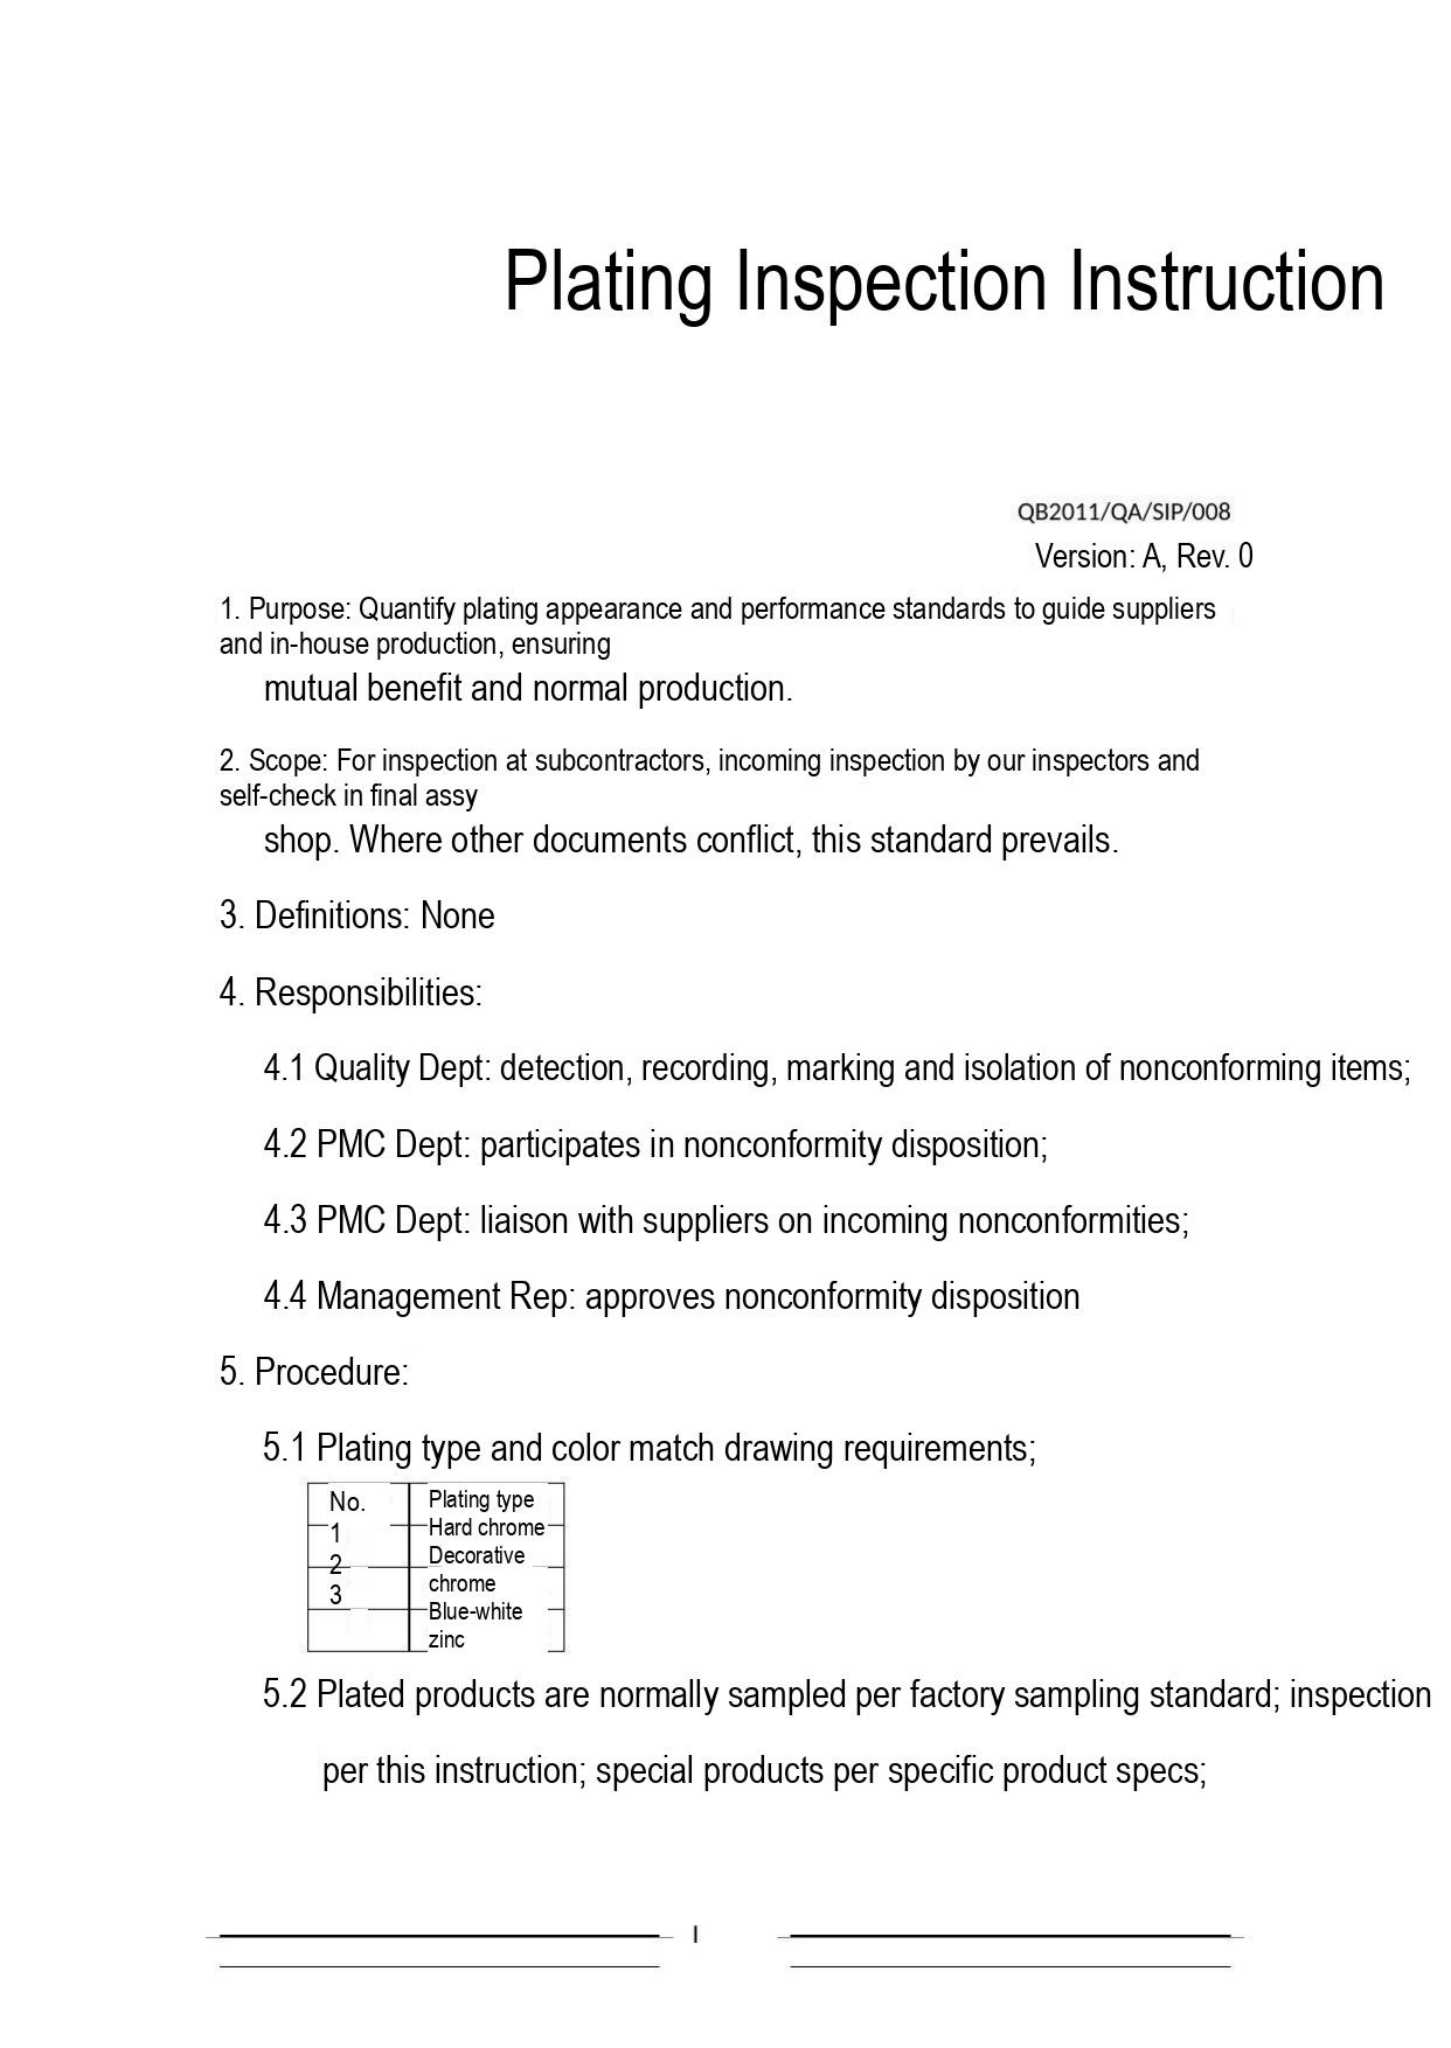# Plating Inspection Instruction

QB2011/QA/SIP/008
Version: A, Rev. 0

1. Purpose: Quantify plating appearance and performance standards to guide suppliers and in-house production, ensuring
mutual benefit and normal production.

2. Scope: For inspection at subcontractors, incoming inspection by our inspectors and self-check in final assy
shop. Where other documents conflict, this standard prevails.

3. Definitions: None

4. Responsibilities:

4.1 Quality Dept: detection, recording, marking and isolation of nonconforming items;

4.2 PMC Dept: participates in nonconformity disposition;

4.3 PMC Dept: liaison with suppliers on incoming nonconformities;

4.4 Management Rep: approves nonconformity disposition

5. Procedure:

5.1 Plating type and color match drawing requirements;

| No. | Plating type |
|---|---|
| 1 | Hard chrome |
| 2 | Decorative chrome |
| 3 | Blue-white zinc |

5.2 Plated products are normally sampled per factory sampling standard; inspection per this instruction; special products per specific product specs;

I
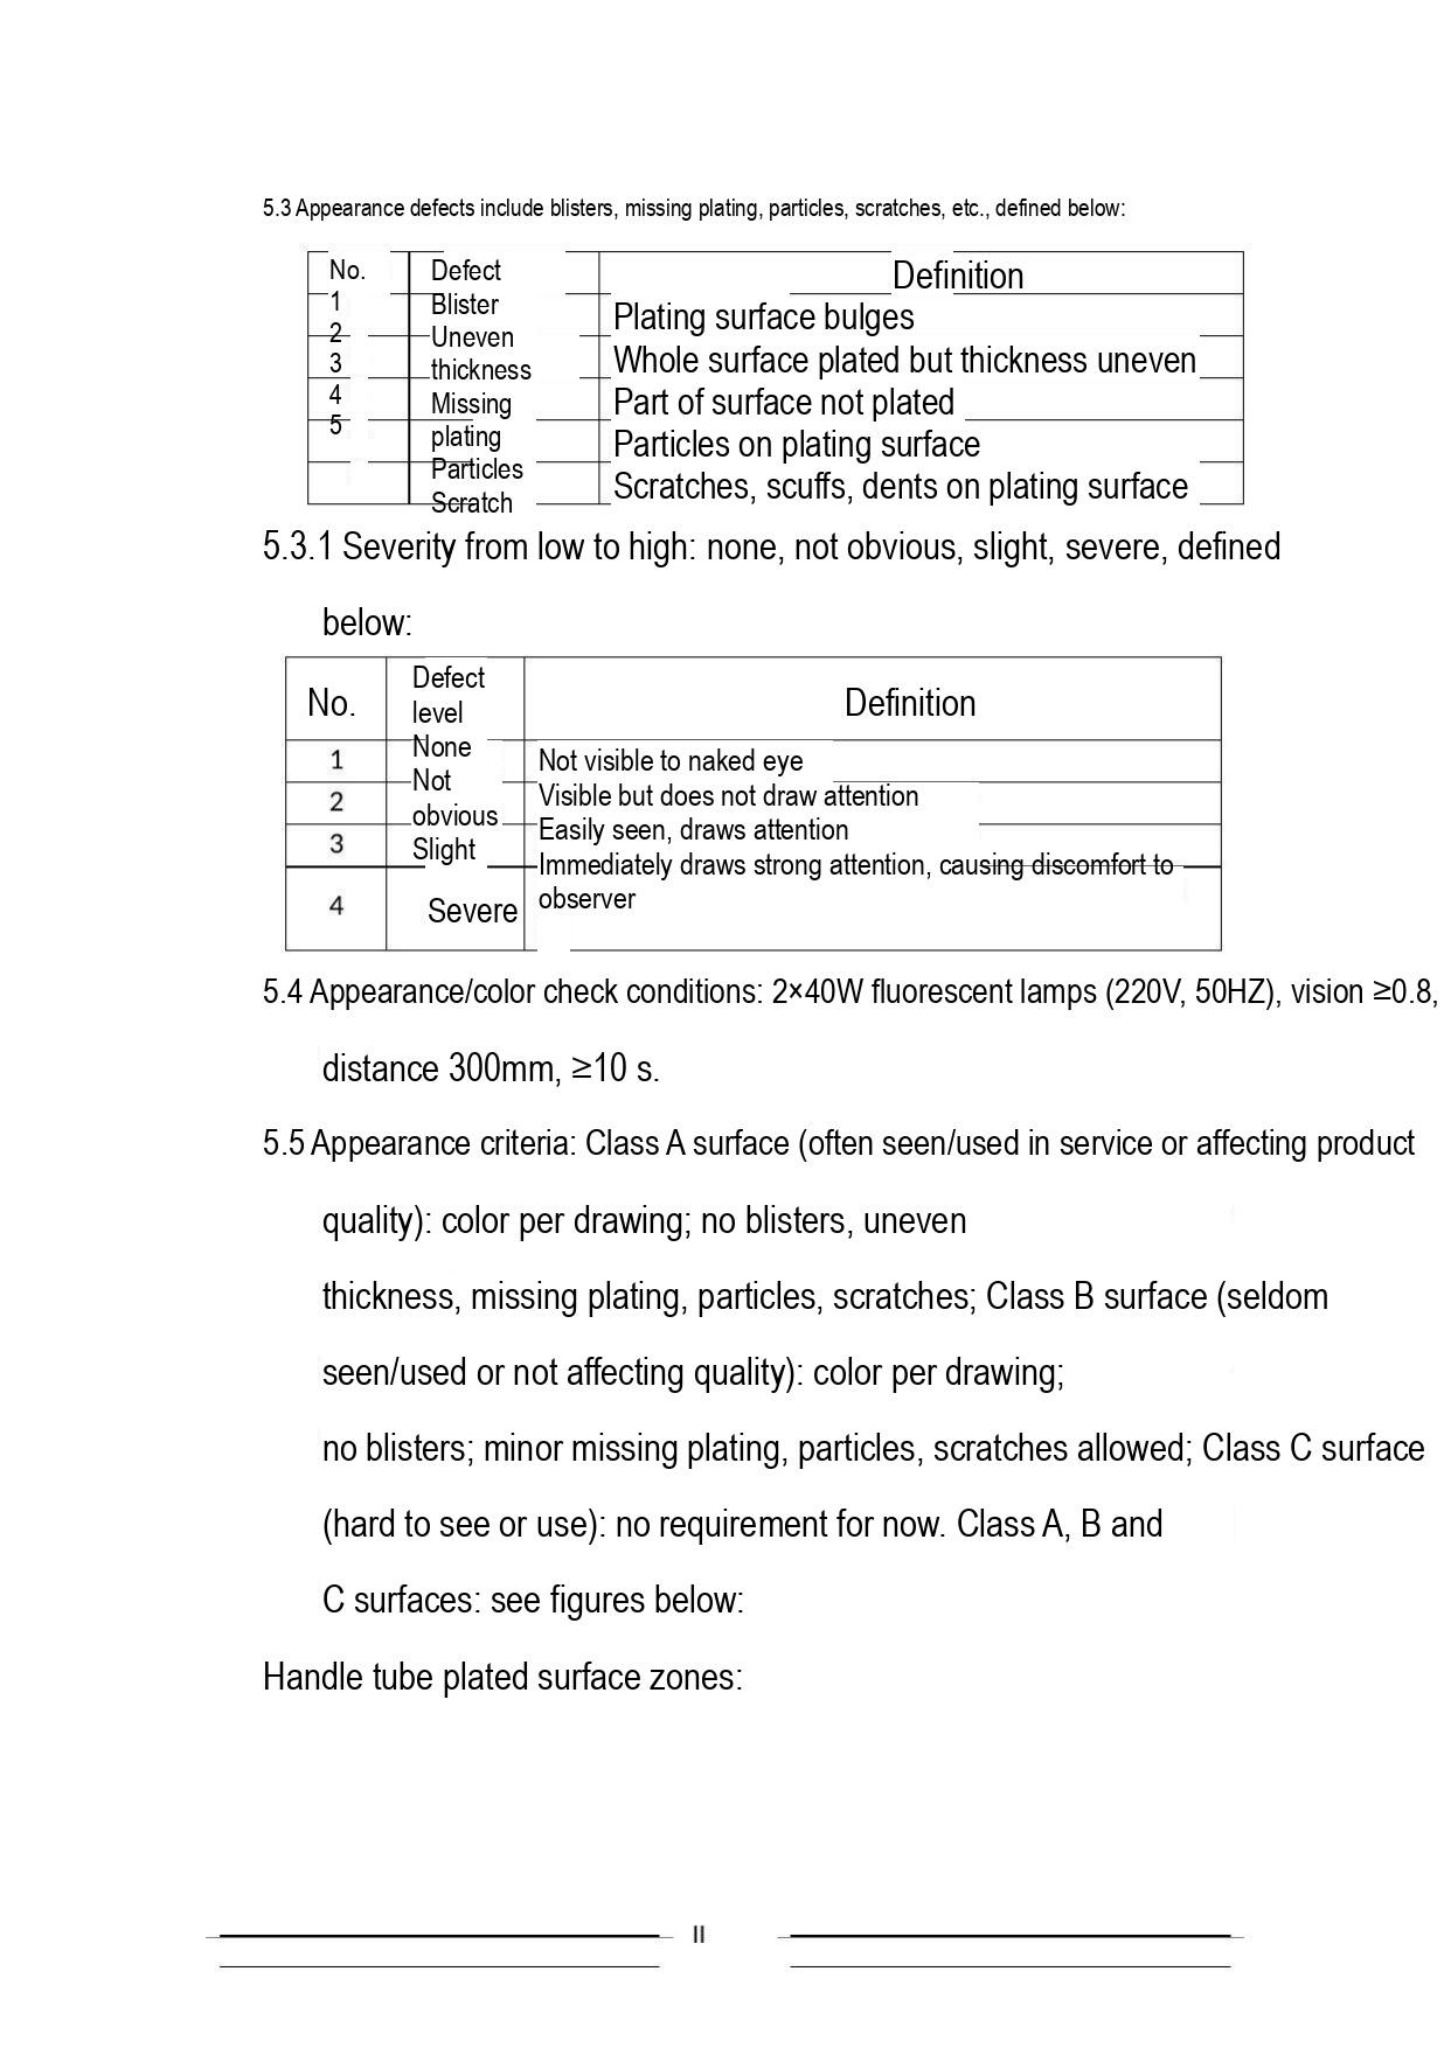5.3 Appearance defects include blisters, missing plating, particles, scratches, etc., defined below:

| No. | Defect | Definition |
|---|---|---|
| 1 | Blister | Plating surface bulges |
| 2 | Uneven thickness | Whole surface plated but thickness uneven |
| 3 | Missing plating | Part of surface not plated |
| 4 | Particles | Particles on plating surface |
| 5 | Scratch | Scratches, scuffs, dents on plating surface |

5.3.1 Severity from low to high: none, not obvious, slight, severe, defined below:

| No. | Defect level | Definition |
|---|---|---|
| 1 | None | Not visible to naked eye |
| 2 | Not obvious | Visible but does not draw attention |
| 3 | Slight | Easily seen, draws attention |
| 4 | Severe | Immediately draws strong attention, causing discomfort to observer |

5.4 Appearance/color check conditions: 2×40W fluorescent lamps (220V, 50HZ), vision ≥0.8, distance 300mm, ≥10 s.

5.5 Appearance criteria: Class A surface (often seen/used in service or affecting product quality): color per drawing; no blisters, uneven thickness, missing plating, particles, scratches; Class B surface (seldom seen/used or not affecting quality): color per drawing; no blisters; minor missing plating, particles, scratches allowed; Class C surface (hard to see or use): no requirement for now. Class A, B and C surfaces: see figures below:

Handle tube plated surface zones:

II
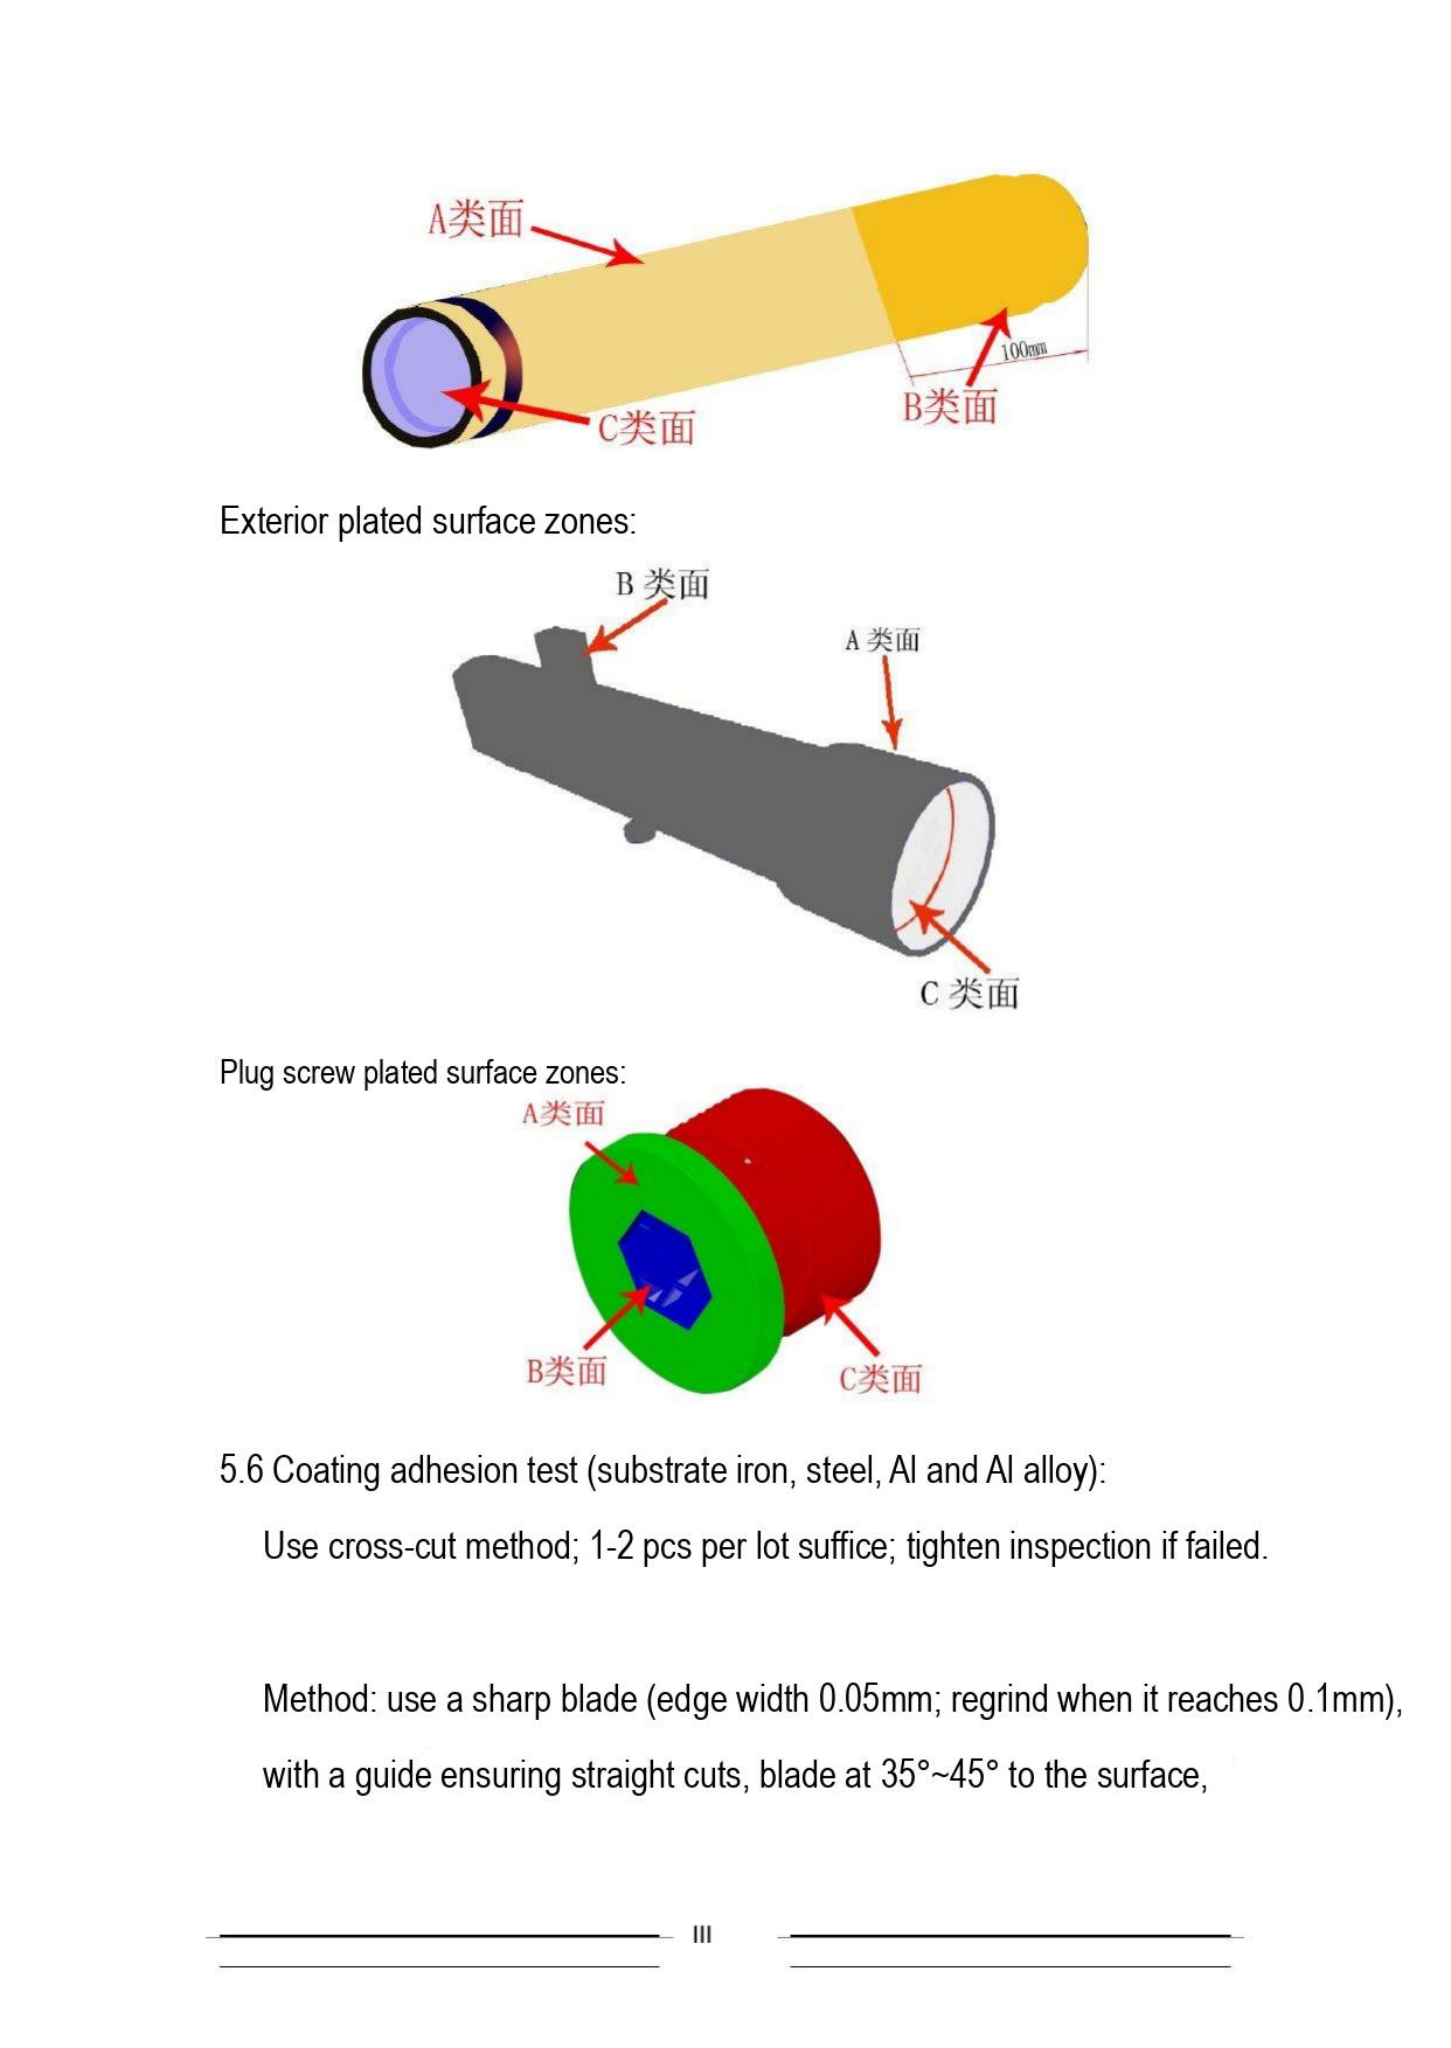A类面

100mm

C类面

B类面

Exterior plated surface zones:

B 类面

A 类面

C 类面

Plug screw plated surface zones:

A类面

B类面

C类面

5.6 Coating adhesion test (substrate iron, steel, Al and Al alloy):

Use cross-cut method; 1-2 pcs per lot suffice; tighten inspection if failed.

Method: use a sharp blade (edge width 0.05mm; regrind when it reaches 0.1mm), with a guide ensuring straight cuts, blade at 35°~45° to the surface,

III
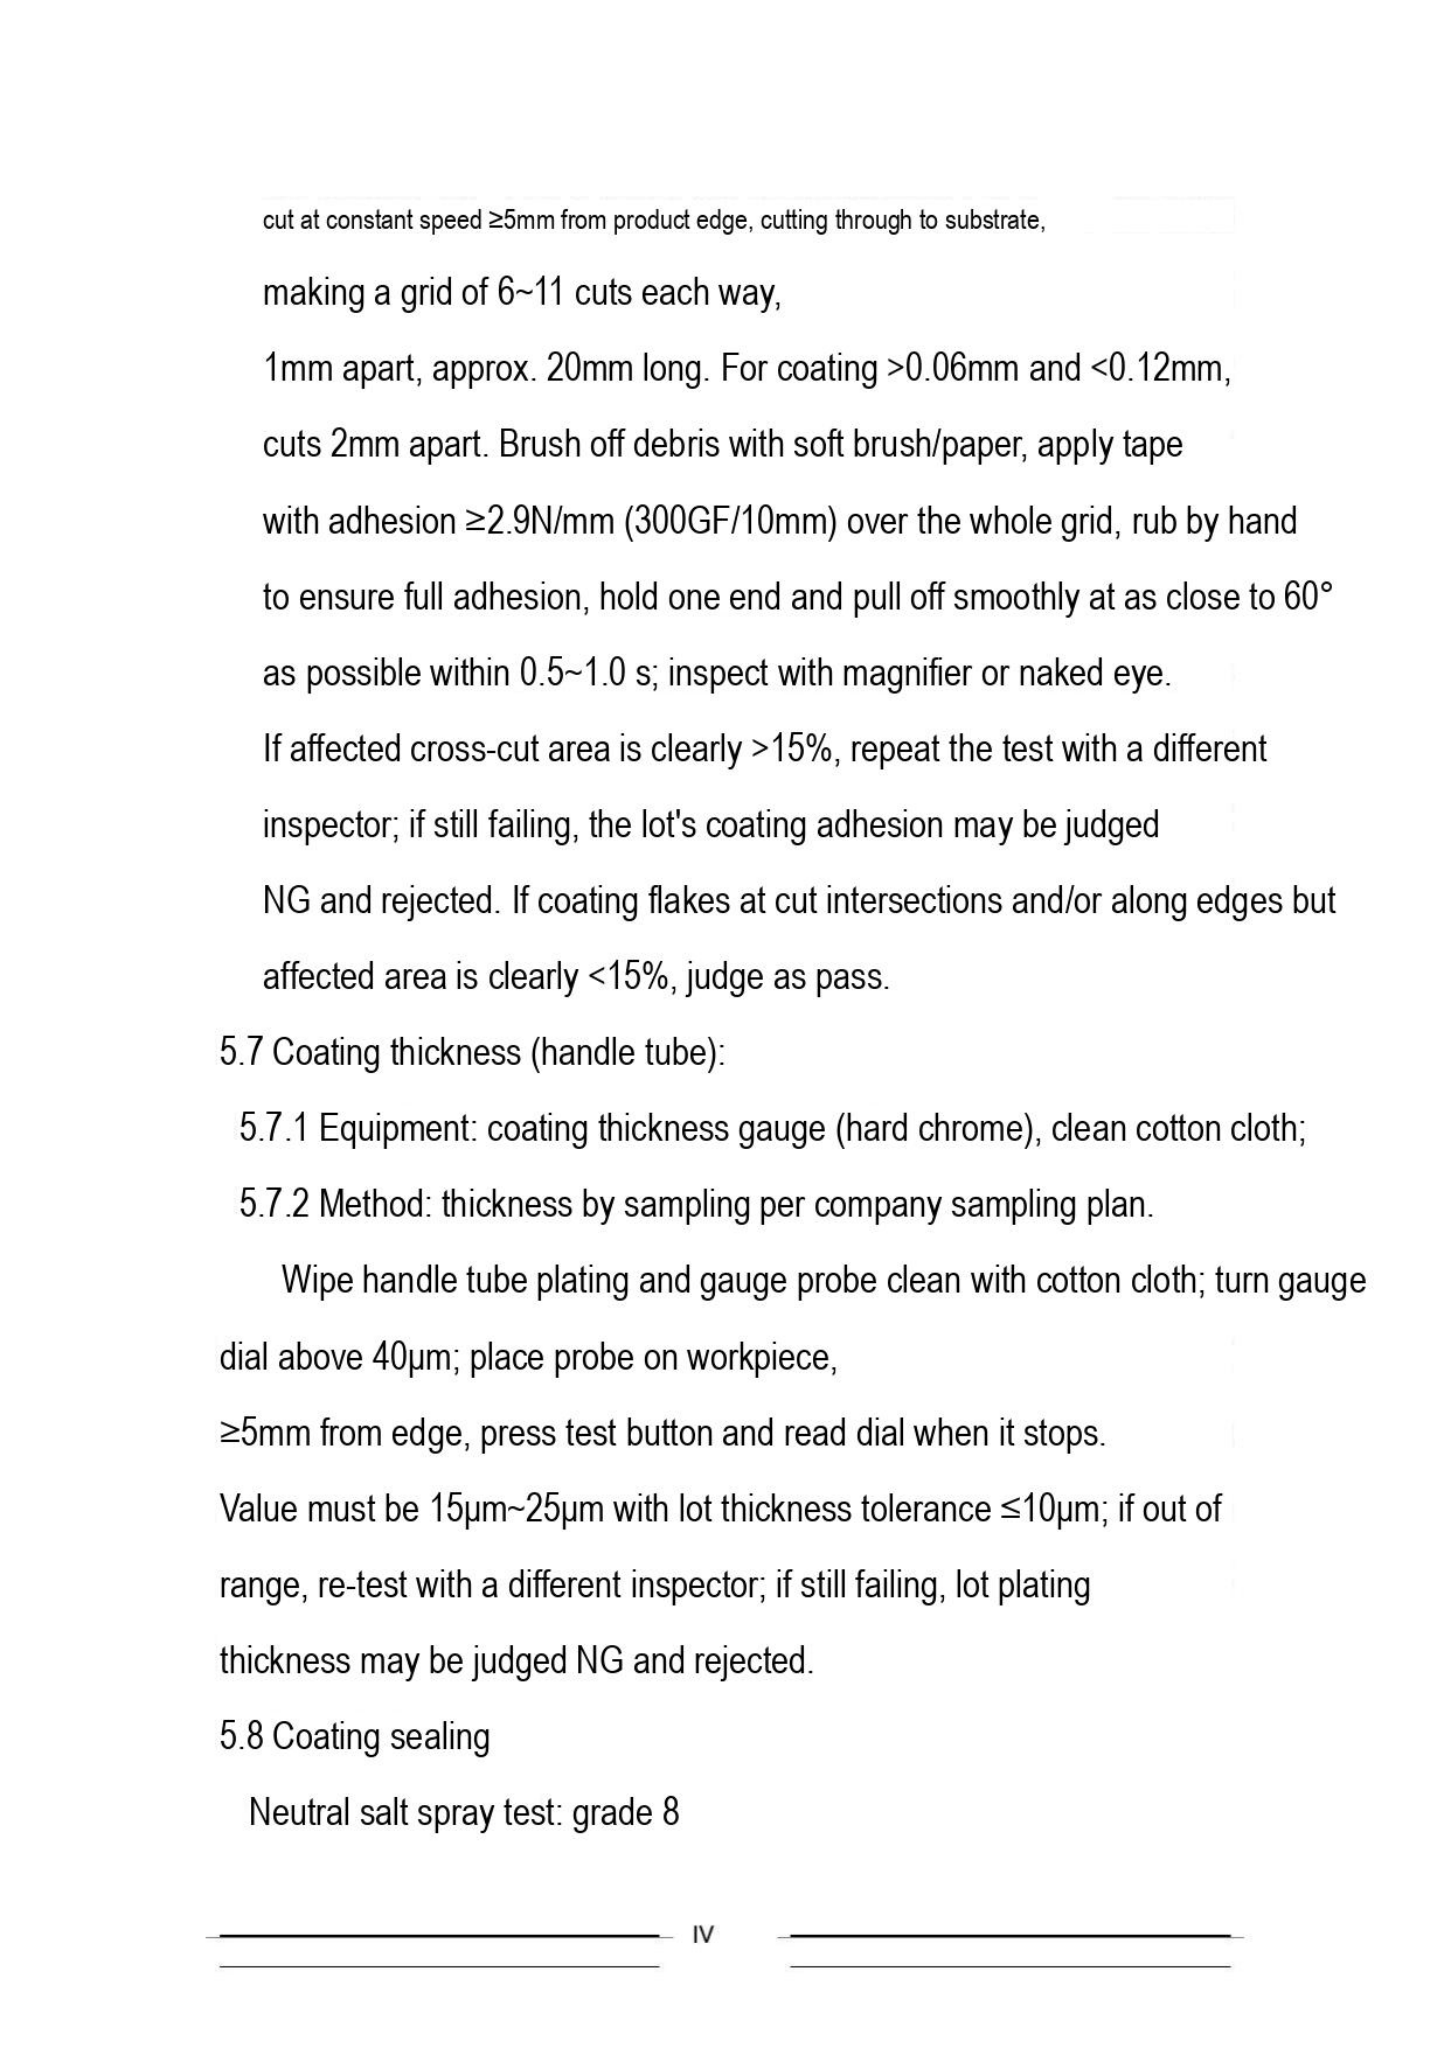cut at constant speed ≥5mm from product edge, cutting through to substrate,

making a grid of 6~11 cuts each way,

1mm apart, approx. 20mm long. For coating >0.06mm and <0.12mm,

cuts 2mm apart. Brush off debris with soft brush/paper, apply tape

with adhesion ≥2.9N/mm (300GF/10mm) over the whole grid, rub by hand

to ensure full adhesion, hold one end and pull off smoothly at as close to 60°

as possible within 0.5~1.0 s; inspect with magnifier or naked eye.

If affected cross-cut area is clearly >15%, repeat the test with a different

inspector; if still failing, the lot's coating adhesion may be judged

NG and rejected. If coating flakes at cut intersections and/or along edges but

affected area is clearly <15%, judge as pass.

5.7 Coating thickness (handle tube):

5.7.1 Equipment: coating thickness gauge (hard chrome), clean cotton cloth;

5.7.2 Method: thickness by sampling per company sampling plan.

Wipe handle tube plating and gauge probe clean with cotton cloth; turn gauge

dial above 40μm; place probe on workpiece,

≥5mm from edge, press test button and read dial when it stops.

Value must be 15μm~25μm with lot thickness tolerance ≤10μm; if out of

range, re-test with a different inspector; if still failing, lot plating

thickness may be judged NG and rejected.

5.8 Coating sealing

Neutral salt spray test: grade 8

IV
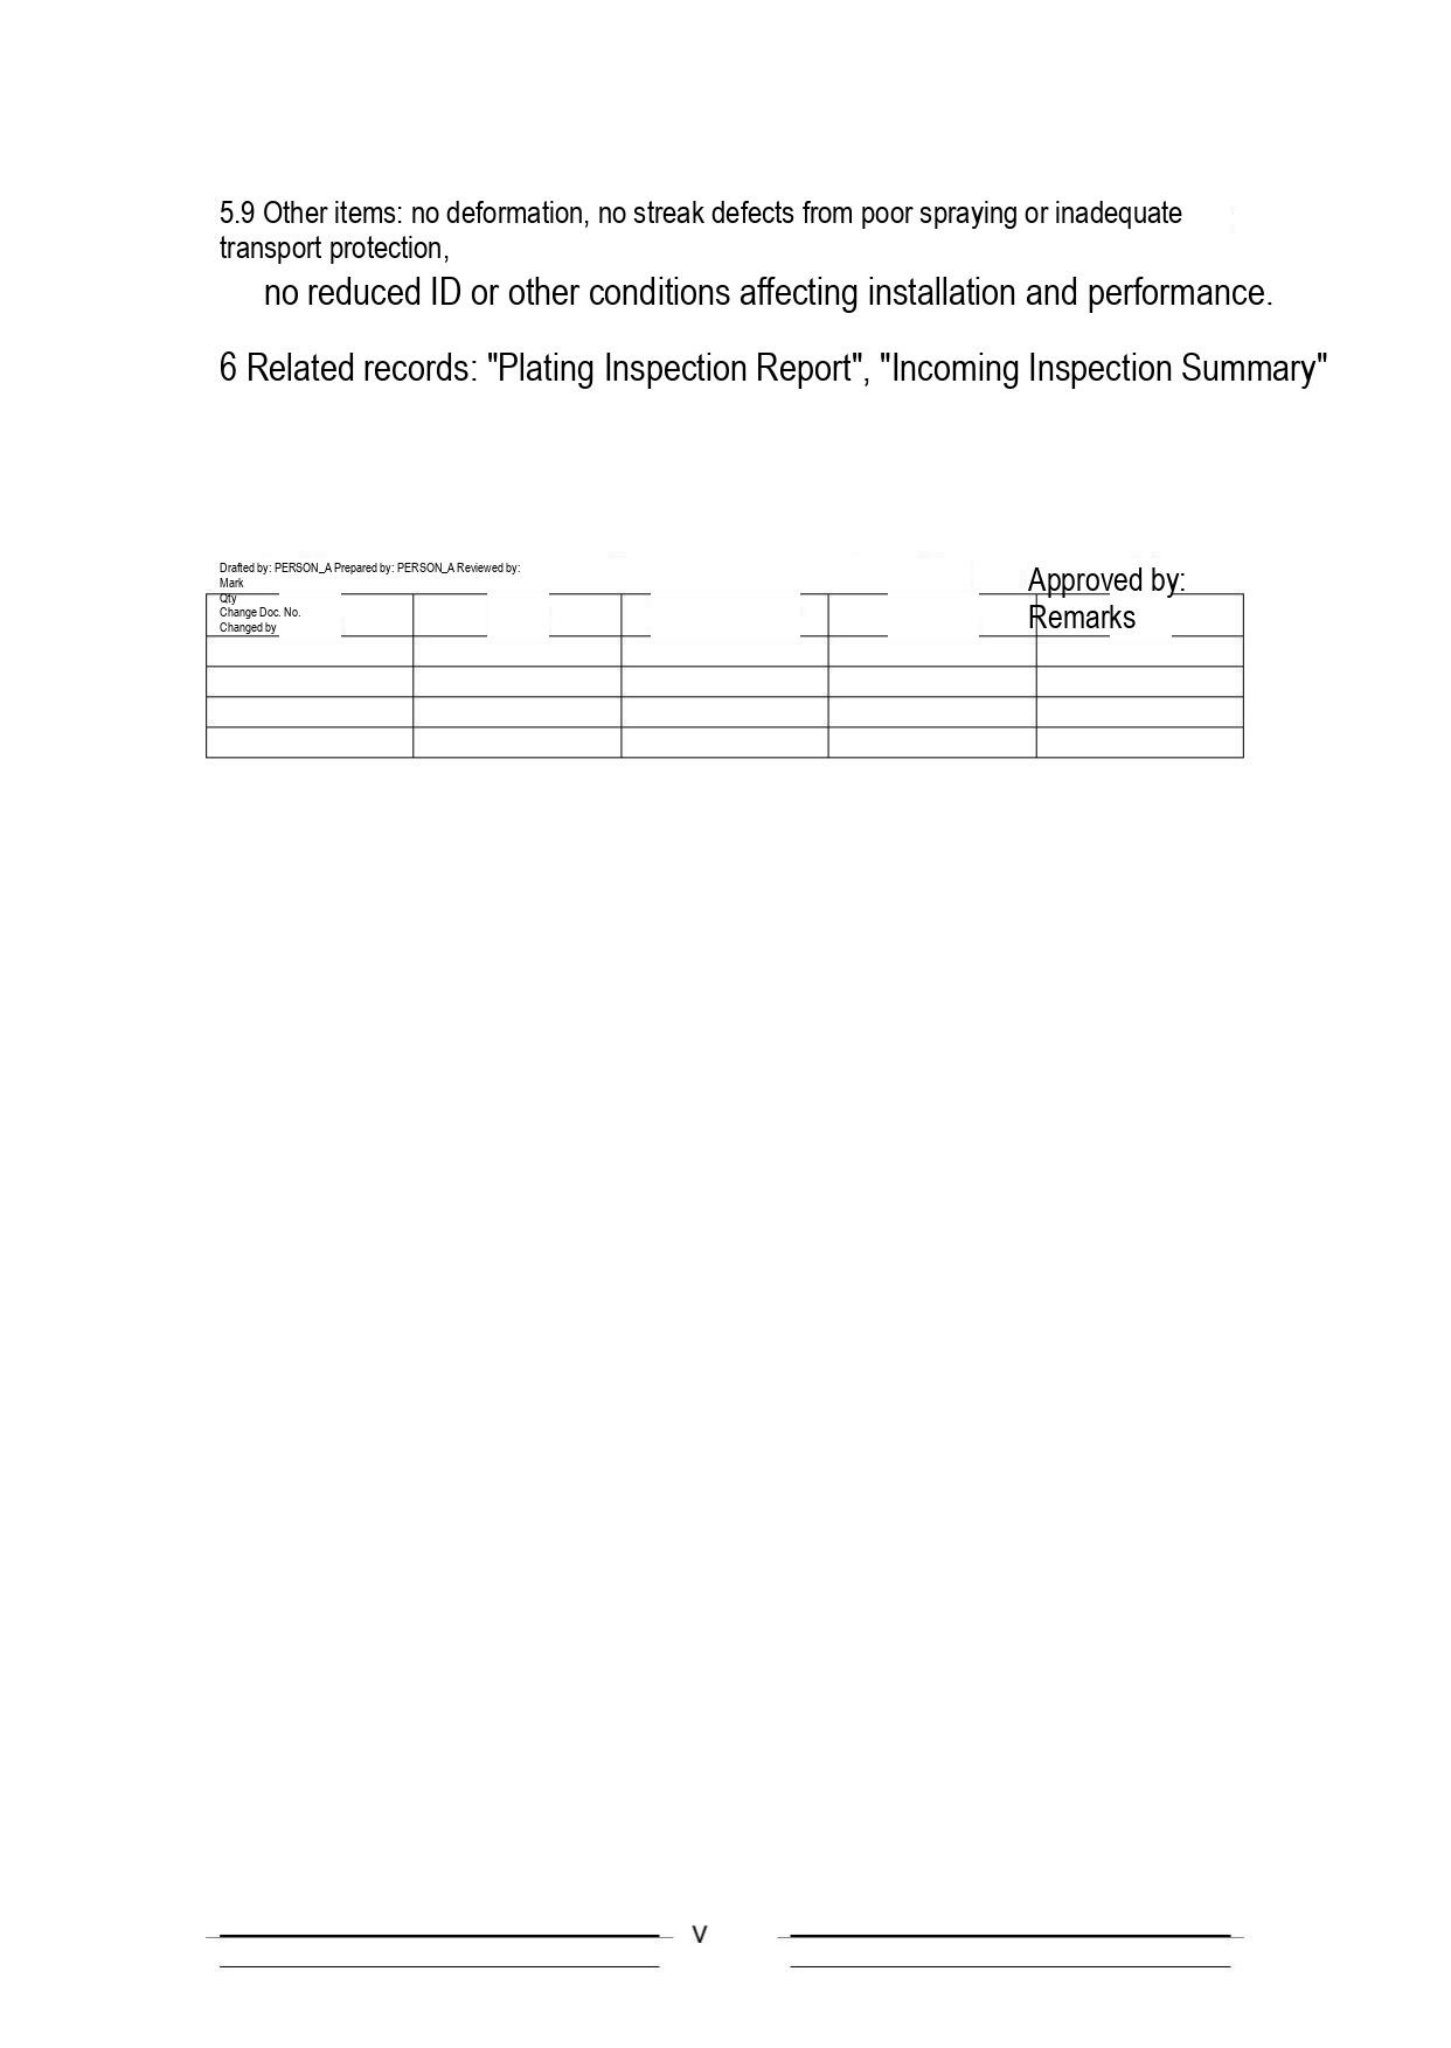5.9 Other items: no deformation, no streak defects from poor spraying or inadequate transport protection,

no reduced ID or other conditions affecting installation and performance.

6 Related records: "Plating Inspection Report", "Incoming Inspection Summary"

Drafted by: PERSON_A Prepared by: PERSON_A Reviewed by:

Approved by:

| Mark<br>Qty<br>Change Doc. No.<br>Changed by | | | | Remarks |
|---|---|---|---|---|
| | | | | |
| | | | | |
| | | | | |
| | | | | |

V